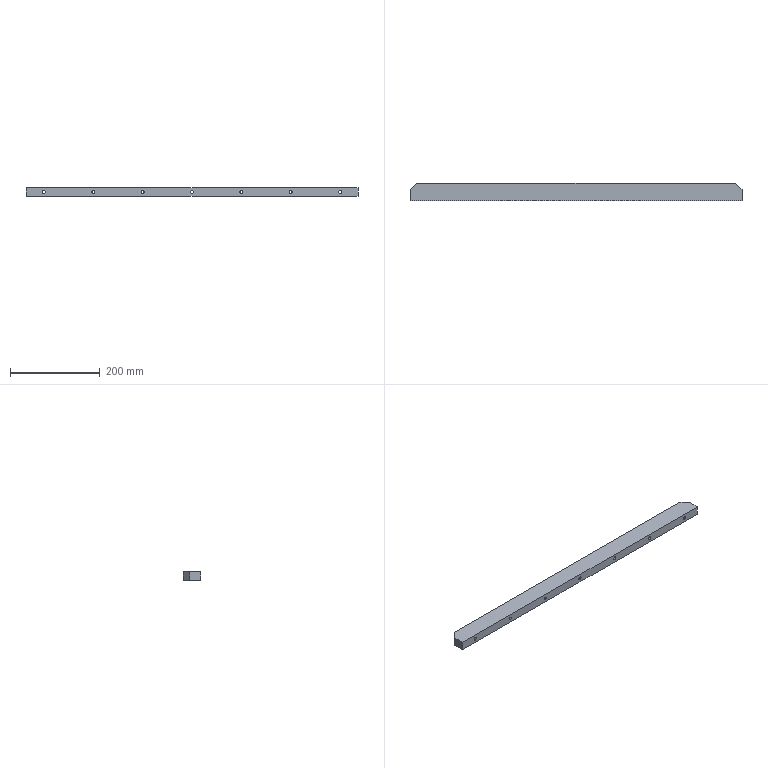Part | SolidWorks | features BaseBody 1 | 1 solid | 43 faces | box 740 x 40 x 20 mm | volume 575026 mm3 | cylinder 28 | plane 15 | commonest cylinder face diameters 6.6 x14 11 x14
STEP:
#1=CARTESIAN_POINT('',(-330.,33.2,-5.5));
#2=VERTEX_POINT('',#1);
#3=CARTESIAN_POINT('',(-330.,33.2,5.5));
#4=VERTEX_POINT('',#3);
#5=CARTESIAN_POINT('',(-330.,33.2,0.));
#6=DIRECTION('',(0.,1.,0.));
#7=DIRECTION('',(0.,0.,1.));
#8=AXIS2_PLACEMENT_3D('',#5,#6,#7);
#9=CIRCLE('',#8,5.5);
#10=EDGE_CURVE('',#2,#4,#9,.T.);
#11=ORIENTED_EDGE('',*,*,#10,.F.);
#12=CARTESIAN_POINT('',(-330.,40.,-5.5));
#13=VERTEX_POINT('',#12);
#14=CARTESIAN_POINT('',(-330.,40.,-5.5));
#15=DIRECTION('',(0.,1.,0.));
#16=VECTOR('',#15,1000.);
#17=LINE('',#14,#16);
#18=EDGE_CURVE('',#2,#13,#17,.T.);
#19=ORIENTED_EDGE('',*,*,#18,.T.);
#20=CARTESIAN_POINT('',(-330.,40.,5.5));
#21=VERTEX_POINT('',#20);
#22=CARTESIAN_POINT('',(-330.,40.,0.));
#23=DIRECTION('',(0.,1.,0.));
#24=DIRECTION('',(0.,0.,1.));
#25=AXIS2_PLACEMENT_3D('',#22,#23,#24);
#26=CIRCLE('',#25,5.5);
#27=EDGE_CURVE('',#13,#21,#26,.T.);
#28=ORIENTED_EDGE('',*,*,#27,.T.);
#29=CARTESIAN_POINT('',(-330.,40.,5.5));
#30=DIRECTION('',(0.,1.,0.));
#31=VECTOR('',#30,1000.);
#32=LINE('',#29,#31);
#33=EDGE_CURVE('',#4,#21,#32,.T.);
#34=ORIENTED_EDGE('',*,*,#33,.F.);
#35=EDGE_LOOP('',(#11,#19,#28,#34));
#36=FACE_OUTER_BOUND('',#35,.T.);
#37=CARTESIAN_POINT('',(-330.,40.,0.));
#38=DIRECTION('',(0.,1.,0.));
#39=DIRECTION('',(0.,0.,1.));
#40=AXIS2_PLACEMENT_3D('',#37,#38,#39);
#41=CYLINDRICAL_SURFACE('',#40,5.5);
#42=ADVANCED_FACE('',(#36),#41,.F.);
#43=CARTESIAN_POINT('',(-330.,0.,3.3));
#44=VERTEX_POINT('',#43);
#45=CARTESIAN_POINT('',(-330.,0.,-3.3));
#46=VERTEX_POINT('',#45);
#47=CARTESIAN_POINT('',(-330.,0.,0.));
#48=DIRECTION('',(0.,-1.,0.));
#49=DIRECTION('',(0.,0.,-1.));
#50=AXIS2_PLACEMENT_3D('',#47,#48,#49);
#51=CIRCLE('',#50,3.3);
#52=EDGE_CURVE('',#44,#46,#51,.T.);
#53=ORIENTED_EDGE('',*,*,#52,.T.);
#54=CARTESIAN_POINT('',(-330.,33.2,-3.3));
#55=VERTEX_POINT('',#54);
#56=CARTESIAN_POINT('',(-330.,40.,-3.3));
#57=DIRECTION('',(0.,1.,0.));
#58=VECTOR('',#57,1000.);
#59=LINE('',#56,#58);
#60=EDGE_CURVE('',#46,#55,#59,.T.);
#61=ORIENTED_EDGE('',*,*,#60,.T.);
#62=CARTESIAN_POINT('',(-330.,33.2,3.3));
#63=VERTEX_POINT('',#62);
#64=CARTESIAN_POINT('',(-330.,33.2,0.));
#65=DIRECTION('',(0.,1.,0.));
#66=DIRECTION('',(0.,0.,1.));
#67=AXIS2_PLACEMENT_3D('',#64,#65,#66);
#68=CIRCLE('',#67,3.3);
#69=EDGE_CURVE('',#55,#63,#68,.T.);
#70=ORIENTED_EDGE('',*,*,#69,.T.);
#71=CARTESIAN_POINT('',(-330.,40.,3.3));
#72=DIRECTION('',(0.,1.,0.));
#73=VECTOR('',#72,1000.);
#74=LINE('',#71,#73);
#75=EDGE_CURVE('',#44,#63,#74,.T.);
#76=ORIENTED_EDGE('',*,*,#75,.F.);
#77=EDGE_LOOP('',(#53,#61,#70,#76));
#78=FACE_OUTER_BOUND('',#77,.T.);
#79=CARTESIAN_POINT('',(-330.,40.,0.));
#80=DIRECTION('',(0.,1.,0.));
#81=DIRECTION('',(0.,0.,1.));
#82=AXIS2_PLACEMENT_3D('',#79,#80,#81);
#83=CYLINDRICAL_SURFACE('',#82,3.3);
#84=ADVANCED_FACE('',(#78),#83,.F.);
#85=CARTESIAN_POINT('',(-220.,33.2,-5.5));
#86=VERTEX_POINT('',#85);
#87=CARTESIAN_POINT('',(-220.,33.2,5.5));
#88=VERTEX_POINT('',#87);
#89=CARTESIAN_POINT('',(-220.,33.2,0.));
#90=DIRECTION('',(0.,1.,0.));
#91=DIRECTION('',(0.,0.,1.));
#92=AXIS2_PLACEMENT_3D('',#89,#90,#91);
#93=CIRCLE('',#92,5.5);
#94=EDGE_CURVE('',#86,#88,#93,.T.);
#95=ORIENTED_EDGE('',*,*,#94,.F.);
#96=CARTESIAN_POINT('',(-220.,40.,-5.5));
#97=VERTEX_POINT('',#96);
#98=CARTESIAN_POINT('',(-220.,40.,-5.5));
#99=DIRECTION('',(0.,1.,0.));
#100=VECTOR('',#99,1000.);
#101=LINE('',#98,#100);
#102=EDGE_CURVE('',#86,#97,#101,.T.);
#103=ORIENTED_EDGE('',*,*,#102,.T.);
#104=CARTESIAN_POINT('',(-220.,40.,5.5));
#105=VERTEX_POINT('',#104);
#106=CARTESIAN_POINT('',(-220.,40.,0.));
#107=DIRECTION('',(0.,1.,0.));
#108=DIRECTION('',(0.,0.,1.));
#109=AXIS2_PLACEMENT_3D('',#106,#107,#108);
#110=CIRCLE('',#109,5.5);
#111=EDGE_CURVE('',#97,#105,#110,.T.);
#112=ORIENTED_EDGE('',*,*,#111,.T.);
#113=CARTESIAN_POINT('',(-220.,40.,5.5));
#114=DIRECTION('',(0.,1.,0.));
#115=VECTOR('',#114,1000.);
#116=LINE('',#113,#115);
#117=EDGE_CURVE('',#88,#105,#116,.T.);
#118=ORIENTED_EDGE('',*,*,#117,.F.);
#119=EDGE_LOOP('',(#95,#103,#112,#118));
#120=FACE_OUTER_BOUND('',#119,.T.);
#121=CARTESIAN_POINT('',(-220.,40.,0.));
#122=DIRECTION('',(0.,1.,0.));
#123=DIRECTION('',(0.,0.,1.));
#124=AXIS2_PLACEMENT_3D('',#121,#122,#123);
#125=CYLINDRICAL_SURFACE('',#124,5.5);
#126=ADVANCED_FACE('',(#120),#125,.F.);
#127=CARTESIAN_POINT('',(-220.,0.,3.3));
#128=VERTEX_POINT('',#127);
#129=CARTESIAN_POINT('',(-220.,0.,-3.3));
#130=VERTEX_POINT('',#129);
#131=CARTESIAN_POINT('',(-220.,0.,0.));
#132=DIRECTION('',(0.,-1.,0.));
#133=DIRECTION('',(0.,0.,-1.));
#134=AXIS2_PLACEMENT_3D('',#131,#132,#133);
#135=CIRCLE('',#134,3.3);
#136=EDGE_CURVE('',#128,#130,#135,.T.);
#137=ORIENTED_EDGE('',*,*,#136,.T.);
#138=CARTESIAN_POINT('',(-220.,33.2,-3.3));
#139=VERTEX_POINT('',#138);
#140=CARTESIAN_POINT('',(-220.,40.,-3.3));
#141=DIRECTION('',(0.,1.,0.));
#142=VECTOR('',#141,1000.);
#143=LINE('',#140,#142);
#144=EDGE_CURVE('',#130,#139,#143,.T.);
#145=ORIENTED_EDGE('',*,*,#144,.T.);
#146=CARTESIAN_POINT('',(-220.,33.2,3.3));
#147=VERTEX_POINT('',#146);
#148=CARTESIAN_POINT('',(-220.,33.2,0.));
#149=DIRECTION('',(0.,1.,0.));
#150=DIRECTION('',(0.,0.,1.));
#151=AXIS2_PLACEMENT_3D('',#148,#149,#150);
#152=CIRCLE('',#151,3.3);
#153=EDGE_CURVE('',#139,#147,#152,.T.);
#154=ORIENTED_EDGE('',*,*,#153,.T.);
#155=CARTESIAN_POINT('',(-220.,40.,3.3));
#156=DIRECTION('',(0.,1.,0.));
#157=VECTOR('',#156,1000.);
#158=LINE('',#155,#157);
#159=EDGE_CURVE('',#128,#147,#158,.T.);
#160=ORIENTED_EDGE('',*,*,#159,.F.);
#161=EDGE_LOOP('',(#137,#145,#154,#160));
#162=FACE_OUTER_BOUND('',#161,.T.);
#163=CARTESIAN_POINT('',(-220.,40.,0.));
#164=DIRECTION('',(0.,1.,0.));
#165=DIRECTION('',(0.,0.,1.));
#166=AXIS2_PLACEMENT_3D('',#163,#164,#165);
#167=CYLINDRICAL_SURFACE('',#166,3.3);
#168=ADVANCED_FACE('',(#162),#167,.F.);
#169=CARTESIAN_POINT('',(-110.,33.2,-5.5));
#170=VERTEX_POINT('',#169);
#171=CARTESIAN_POINT('',(-110.,33.2,5.5));
#172=VERTEX_POINT('',#171);
#173=CARTESIAN_POINT('',(-110.,33.2,0.));
#174=DIRECTION('',(0.,1.,0.));
#175=DIRECTION('',(0.,0.,1.));
#176=AXIS2_PLACEMENT_3D('',#173,#174,#175);
#177=CIRCLE('',#176,5.5);
#178=EDGE_CURVE('',#170,#172,#177,.T.);
#179=ORIENTED_EDGE('',*,*,#178,.F.);
#180=CARTESIAN_POINT('',(-110.,40.,-5.5));
#181=VERTEX_POINT('',#180);
#182=CARTESIAN_POINT('',(-110.,40.,-5.5));
#183=DIRECTION('',(0.,1.,0.));
#184=VECTOR('',#183,1000.);
#185=LINE('',#182,#184);
#186=EDGE_CURVE('',#170,#181,#185,.T.);
#187=ORIENTED_EDGE('',*,*,#186,.T.);
#188=CARTESIAN_POINT('',(-110.,40.,5.5));
#189=VERTEX_POINT('',#188);
#190=CARTESIAN_POINT('',(-110.,40.,0.));
#191=DIRECTION('',(0.,1.,0.));
#192=DIRECTION('',(0.,0.,1.));
#193=AXIS2_PLACEMENT_3D('',#190,#191,#192);
#194=CIRCLE('',#193,5.5);
#195=EDGE_CURVE('',#181,#189,#194,.T.);
#196=ORIENTED_EDGE('',*,*,#195,.T.);
#197=CARTESIAN_POINT('',(-110.,40.,5.5));
#198=DIRECTION('',(0.,1.,0.));
#199=VECTOR('',#198,1000.);
#200=LINE('',#197,#199);
#201=EDGE_CURVE('',#172,#189,#200,.T.);
#202=ORIENTED_EDGE('',*,*,#201,.F.);
#203=EDGE_LOOP('',(#179,#187,#196,#202));
#204=FACE_OUTER_BOUND('',#203,.T.);
#205=CARTESIAN_POINT('',(-110.,40.,0.));
#206=DIRECTION('',(0.,1.,0.));
#207=DIRECTION('',(0.,0.,1.));
#208=AXIS2_PLACEMENT_3D('',#205,#206,#207);
#209=CYLINDRICAL_SURFACE('',#208,5.5);
#210=ADVANCED_FACE('',(#204),#209,.F.);
#211=CARTESIAN_POINT('',(-110.,0.,3.3));
#212=VERTEX_POINT('',#211);
#213=CARTESIAN_POINT('',(-110.,0.,-3.3));
#214=VERTEX_POINT('',#213);
#215=CARTESIAN_POINT('',(-110.,0.,0.));
#216=DIRECTION('',(0.,-1.,0.));
#217=DIRECTION('',(0.,0.,-1.));
#218=AXIS2_PLACEMENT_3D('',#215,#216,#217);
#219=CIRCLE('',#218,3.3);
#220=EDGE_CURVE('',#212,#214,#219,.T.);
#221=ORIENTED_EDGE('',*,*,#220,.T.);
#222=CARTESIAN_POINT('',(-110.,33.2,-3.3));
#223=VERTEX_POINT('',#222);
#224=CARTESIAN_POINT('',(-110.,40.,-3.3));
#225=DIRECTION('',(0.,1.,0.));
#226=VECTOR('',#225,1000.);
#227=LINE('',#224,#226);
#228=EDGE_CURVE('',#214,#223,#227,.T.);
#229=ORIENTED_EDGE('',*,*,#228,.T.);
#230=CARTESIAN_POINT('',(-110.,33.2,3.3));
#231=VERTEX_POINT('',#230);
#232=CARTESIAN_POINT('',(-110.,33.2,0.));
#233=DIRECTION('',(0.,1.,0.));
#234=DIRECTION('',(0.,0.,1.));
#235=AXIS2_PLACEMENT_3D('',#232,#233,#234);
#236=CIRCLE('',#235,3.3);
#237=EDGE_CURVE('',#223,#231,#236,.T.);
#238=ORIENTED_EDGE('',*,*,#237,.T.);
#239=CARTESIAN_POINT('',(-110.,40.,3.3));
#240=DIRECTION('',(0.,1.,0.));
#241=VECTOR('',#240,1000.);
#242=LINE('',#239,#241);
#243=EDGE_CURVE('',#212,#231,#242,.T.);
#244=ORIENTED_EDGE('',*,*,#243,.F.);
#245=EDGE_LOOP('',(#221,#229,#238,#244));
#246=FACE_OUTER_BOUND('',#245,.T.);
#247=CARTESIAN_POINT('',(-110.,40.,0.));
#248=DIRECTION('',(0.,1.,0.));
#249=DIRECTION('',(0.,0.,1.));
#250=AXIS2_PLACEMENT_3D('',#247,#248,#249);
#251=CYLINDRICAL_SURFACE('',#250,3.3);
#252=ADVANCED_FACE('',(#246),#251,.F.);
#253=CARTESIAN_POINT('',(0.,33.2,-5.5));
#254=VERTEX_POINT('',#253);
#255=CARTESIAN_POINT('',(0.,33.2,5.5));
#256=VERTEX_POINT('',#255);
#257=CARTESIAN_POINT('',(0.,33.2,0.));
#258=DIRECTION('',(0.,1.,0.));
#259=DIRECTION('',(0.,0.,1.));
#260=AXIS2_PLACEMENT_3D('',#257,#258,#259);
#261=CIRCLE('',#260,5.5);
#262=EDGE_CURVE('',#254,#256,#261,.T.);
#263=ORIENTED_EDGE('',*,*,#262,.F.);
#264=CARTESIAN_POINT('',(0.,40.,-5.5));
#265=VERTEX_POINT('',#264);
#266=CARTESIAN_POINT('',(0.,40.,-5.5));
#267=DIRECTION('',(0.,1.,0.));
#268=VECTOR('',#267,1000.);
#269=LINE('',#266,#268);
#270=EDGE_CURVE('',#254,#265,#269,.T.);
#271=ORIENTED_EDGE('',*,*,#270,.T.);
#272=CARTESIAN_POINT('',(0.,40.,5.5));
#273=VERTEX_POINT('',#272);
#274=CARTESIAN_POINT('',(0.,40.,0.));
#275=DIRECTION('',(0.,1.,0.));
#276=DIRECTION('',(0.,0.,1.));
#277=AXIS2_PLACEMENT_3D('',#274,#275,#276);
#278=CIRCLE('',#277,5.5);
#279=EDGE_CURVE('',#265,#273,#278,.T.);
#280=ORIENTED_EDGE('',*,*,#279,.T.);
#281=CARTESIAN_POINT('',(0.,40.,5.5));
#282=DIRECTION('',(0.,1.,0.));
#283=VECTOR('',#282,1000.);
#284=LINE('',#281,#283);
#285=EDGE_CURVE('',#256,#273,#284,.T.);
#286=ORIENTED_EDGE('',*,*,#285,.F.);
#287=EDGE_LOOP('',(#263,#271,#280,#286));
#288=FACE_OUTER_BOUND('',#287,.T.);
#289=CARTESIAN_POINT('',(0.,40.,0.));
#290=DIRECTION('',(0.,1.,0.));
#291=DIRECTION('',(0.,0.,1.));
#292=AXIS2_PLACEMENT_3D('',#289,#290,#291);
#293=CYLINDRICAL_SURFACE('',#292,5.5);
#294=ADVANCED_FACE('',(#288),#293,.F.);
#295=CARTESIAN_POINT('',(0.,0.,3.3));
#296=VERTEX_POINT('',#295);
#297=CARTESIAN_POINT('',(0.,0.,-3.3));
#298=VERTEX_POINT('',#297);
#299=CARTESIAN_POINT('',(0.,0.,0.));
#300=DIRECTION('',(0.,-1.,0.));
#301=DIRECTION('',(0.,0.,-1.));
#302=AXIS2_PLACEMENT_3D('',#299,#300,#301);
#303=CIRCLE('',#302,3.3);
#304=EDGE_CURVE('',#296,#298,#303,.T.);
#305=ORIENTED_EDGE('',*,*,#304,.T.);
#306=CARTESIAN_POINT('',(0.,33.2,-3.3));
#307=VERTEX_POINT('',#306);
#308=CARTESIAN_POINT('',(0.,40.,-3.3));
#309=DIRECTION('',(0.,1.,0.));
#310=VECTOR('',#309,1000.);
#311=LINE('',#308,#310);
#312=EDGE_CURVE('',#298,#307,#311,.T.);
#313=ORIENTED_EDGE('',*,*,#312,.T.);
#314=CARTESIAN_POINT('',(0.,33.2,3.3));
#315=VERTEX_POINT('',#314);
#316=CARTESIAN_POINT('',(0.,33.2,0.));
#317=DIRECTION('',(0.,1.,0.));
#318=DIRECTION('',(0.,0.,1.));
#319=AXIS2_PLACEMENT_3D('',#316,#317,#318);
#320=CIRCLE('',#319,3.3);
#321=EDGE_CURVE('',#307,#315,#320,.T.);
#322=ORIENTED_EDGE('',*,*,#321,.T.);
#323=CARTESIAN_POINT('',(0.,40.,3.3));
#324=DIRECTION('',(0.,1.,0.));
#325=VECTOR('',#324,1000.);
#326=LINE('',#323,#325);
#327=EDGE_CURVE('',#296,#315,#326,.T.);
#328=ORIENTED_EDGE('',*,*,#327,.F.);
#329=EDGE_LOOP('',(#305,#313,#322,#328));
#330=FACE_OUTER_BOUND('',#329,.T.);
#331=CARTESIAN_POINT('',(0.,40.,0.));
#332=DIRECTION('',(0.,1.,0.));
#333=DIRECTION('',(0.,0.,1.));
#334=AXIS2_PLACEMENT_3D('',#331,#332,#333);
#335=CYLINDRICAL_SURFACE('',#334,3.3);
#336=ADVANCED_FACE('',(#330),#335,.F.);
#337=CARTESIAN_POINT('',(110.,33.2,-5.5));
#338=VERTEX_POINT('',#337);
#339=CARTESIAN_POINT('',(110.,33.2,5.5));
#340=VERTEX_POINT('',#339);
#341=CARTESIAN_POINT('',(110.,33.2,0.));
#342=DIRECTION('',(0.,1.,0.));
#343=DIRECTION('',(0.,0.,1.));
#344=AXIS2_PLACEMENT_3D('',#341,#342,#343);
#345=CIRCLE('',#344,5.5);
#346=EDGE_CURVE('',#338,#340,#345,.T.);
#347=ORIENTED_EDGE('',*,*,#346,.F.);
#348=CARTESIAN_POINT('',(110.,40.,-5.5));
#349=VERTEX_POINT('',#348);
#350=CARTESIAN_POINT('',(110.,40.,-5.5));
#351=DIRECTION('',(0.,1.,0.));
#352=VECTOR('',#351,1000.);
#353=LINE('',#350,#352);
#354=EDGE_CURVE('',#338,#349,#353,.T.);
#355=ORIENTED_EDGE('',*,*,#354,.T.);
#356=CARTESIAN_POINT('',(110.,40.,5.5));
#357=VERTEX_POINT('',#356);
#358=CARTESIAN_POINT('',(110.,40.,0.));
#359=DIRECTION('',(0.,1.,0.));
#360=DIRECTION('',(0.,0.,1.));
#361=AXIS2_PLACEMENT_3D('',#358,#359,#360);
#362=CIRCLE('',#361,5.5);
#363=EDGE_CURVE('',#349,#357,#362,.T.);
#364=ORIENTED_EDGE('',*,*,#363,.T.);
#365=CARTESIAN_POINT('',(110.,40.,5.5));
#366=DIRECTION('',(0.,1.,0.));
#367=VECTOR('',#366,1000.);
#368=LINE('',#365,#367);
#369=EDGE_CURVE('',#340,#357,#368,.T.);
#370=ORIENTED_EDGE('',*,*,#369,.F.);
#371=EDGE_LOOP('',(#347,#355,#364,#370));
#372=FACE_OUTER_BOUND('',#371,.T.);
#373=CARTESIAN_POINT('',(110.,40.,0.));
#374=DIRECTION('',(0.,1.,0.));
#375=DIRECTION('',(0.,0.,1.));
#376=AXIS2_PLACEMENT_3D('',#373,#374,#375);
#377=CYLINDRICAL_SURFACE('',#376,5.5);
#378=ADVANCED_FACE('',(#372),#377,.F.);
#379=CARTESIAN_POINT('',(110.,0.,3.3));
#380=VERTEX_POINT('',#379);
#381=CARTESIAN_POINT('',(110.,0.,-3.3));
#382=VERTEX_POINT('',#381);
#383=CARTESIAN_POINT('',(110.,0.,0.));
#384=DIRECTION('',(0.,-1.,0.));
#385=DIRECTION('',(0.,0.,-1.));
#386=AXIS2_PLACEMENT_3D('',#383,#384,#385);
#387=CIRCLE('',#386,3.3);
#388=EDGE_CURVE('',#380,#382,#387,.T.);
#389=ORIENTED_EDGE('',*,*,#388,.T.);
#390=CARTESIAN_POINT('',(110.,33.2,-3.3));
#391=VERTEX_POINT('',#390);
#392=CARTESIAN_POINT('',(110.,40.,-3.3));
#393=DIRECTION('',(0.,1.,0.));
#394=VECTOR('',#393,1000.);
#395=LINE('',#392,#394);
#396=EDGE_CURVE('',#382,#391,#395,.T.);
#397=ORIENTED_EDGE('',*,*,#396,.T.);
#398=CARTESIAN_POINT('',(110.,33.2,3.3));
#399=VERTEX_POINT('',#398);
#400=CARTESIAN_POINT('',(110.,33.2,0.));
#401=DIRECTION('',(0.,1.,0.));
#402=DIRECTION('',(0.,0.,1.));
#403=AXIS2_PLACEMENT_3D('',#400,#401,#402);
#404=CIRCLE('',#403,3.3);
#405=EDGE_CURVE('',#391,#399,#404,.T.);
#406=ORIENTED_EDGE('',*,*,#405,.T.);
#407=CARTESIAN_POINT('',(110.,40.,3.3));
#408=DIRECTION('',(0.,1.,0.));
#409=VECTOR('',#408,1000.);
#410=LINE('',#407,#409);
#411=EDGE_CURVE('',#380,#399,#410,.T.);
#412=ORIENTED_EDGE('',*,*,#411,.F.);
#413=EDGE_LOOP('',(#389,#397,#406,#412));
#414=FACE_OUTER_BOUND('',#413,.T.);
#415=CARTESIAN_POINT('',(110.,40.,0.));
#416=DIRECTION('',(0.,1.,0.));
#417=DIRECTION('',(0.,0.,1.));
#418=AXIS2_PLACEMENT_3D('',#415,#416,#417);
#419=CYLINDRICAL_SURFACE('',#418,3.3);
#420=ADVANCED_FACE('',(#414),#419,.F.);
#421=CARTESIAN_POINT('',(220.,33.2,-5.5));
#422=VERTEX_POINT('',#421);
#423=CARTESIAN_POINT('',(220.,33.2,5.5));
#424=VERTEX_POINT('',#423);
#425=CARTESIAN_POINT('',(220.,33.2,0.));
#426=DIRECTION('',(0.,1.,0.));
#427=DIRECTION('',(0.,0.,1.));
#428=AXIS2_PLACEMENT_3D('',#425,#426,#427);
#429=CIRCLE('',#428,5.5);
#430=EDGE_CURVE('',#422,#424,#429,.T.);
#431=ORIENTED_EDGE('',*,*,#430,.F.);
#432=CARTESIAN_POINT('',(220.,40.,-5.5));
#433=VERTEX_POINT('',#432);
#434=CARTESIAN_POINT('',(220.,40.,-5.5));
#435=DIRECTION('',(0.,1.,0.));
#436=VECTOR('',#435,1000.);
#437=LINE('',#434,#436);
#438=EDGE_CURVE('',#422,#433,#437,.T.);
#439=ORIENTED_EDGE('',*,*,#438,.T.);
#440=CARTESIAN_POINT('',(220.,40.,5.5));
#441=VERTEX_POINT('',#440);
#442=CARTESIAN_POINT('',(220.,40.,0.));
#443=DIRECTION('',(0.,1.,0.));
#444=DIRECTION('',(0.,0.,1.));
#445=AXIS2_PLACEMENT_3D('',#442,#443,#444);
#446=CIRCLE('',#445,5.5);
#447=EDGE_CURVE('',#433,#441,#446,.T.);
#448=ORIENTED_EDGE('',*,*,#447,.T.);
#449=CARTESIAN_POINT('',(220.,40.,5.5));
#450=DIRECTION('',(0.,1.,0.));
#451=VECTOR('',#450,1000.);
#452=LINE('',#449,#451);
#453=EDGE_CURVE('',#424,#441,#452,.T.);
#454=ORIENTED_EDGE('',*,*,#453,.F.);
#455=EDGE_LOOP('',(#431,#439,#448,#454));
#456=FACE_OUTER_BOUND('',#455,.T.);
#457=CARTESIAN_POINT('',(220.,40.,0.));
#458=DIRECTION('',(0.,1.,0.));
#459=DIRECTION('',(0.,0.,1.));
#460=AXIS2_PLACEMENT_3D('',#457,#458,#459);
#461=CYLINDRICAL_SURFACE('',#460,5.5);
#462=ADVANCED_FACE('',(#456),#461,.F.);
#463=CARTESIAN_POINT('',(220.,0.,3.3));
#464=VERTEX_POINT('',#463);
#465=CARTESIAN_POINT('',(220.,0.,-3.3));
#466=VERTEX_POINT('',#465);
#467=CARTESIAN_POINT('',(220.,0.,0.));
#468=DIRECTION('',(0.,-1.,0.));
#469=DIRECTION('',(0.,0.,-1.));
#470=AXIS2_PLACEMENT_3D('',#467,#468,#469);
#471=CIRCLE('',#470,3.3);
#472=EDGE_CURVE('',#464,#466,#471,.T.);
#473=ORIENTED_EDGE('',*,*,#472,.T.);
#474=CARTESIAN_POINT('',(220.,33.2,-3.3));
#475=VERTEX_POINT('',#474);
#476=CARTESIAN_POINT('',(220.,40.,-3.3));
#477=DIRECTION('',(0.,1.,0.));
#478=VECTOR('',#477,1000.);
#479=LINE('',#476,#478);
#480=EDGE_CURVE('',#466,#475,#479,.T.);
#481=ORIENTED_EDGE('',*,*,#480,.T.);
#482=CARTESIAN_POINT('',(220.,33.2,3.3));
#483=VERTEX_POINT('',#482);
#484=CARTESIAN_POINT('',(220.,33.2,0.));
#485=DIRECTION('',(0.,1.,0.));
#486=DIRECTION('',(0.,0.,1.));
#487=AXIS2_PLACEMENT_3D('',#484,#485,#486);
#488=CIRCLE('',#487,3.3);
#489=EDGE_CURVE('',#475,#483,#488,.T.);
#490=ORIENTED_EDGE('',*,*,#489,.T.);
#491=CARTESIAN_POINT('',(220.,40.,3.3));
#492=DIRECTION('',(0.,1.,0.));
#493=VECTOR('',#492,1000.);
#494=LINE('',#491,#493);
#495=EDGE_CURVE('',#464,#483,#494,.T.);
#496=ORIENTED_EDGE('',*,*,#495,.F.);
#497=EDGE_LOOP('',(#473,#481,#490,#496));
#498=FACE_OUTER_BOUND('',#497,.T.);
#499=CARTESIAN_POINT('',(220.,40.,0.));
#500=DIRECTION('',(0.,1.,0.));
#501=DIRECTION('',(0.,0.,1.));
#502=AXIS2_PLACEMENT_3D('',#499,#500,#501);
#503=CYLINDRICAL_SURFACE('',#502,3.3);
#504=ADVANCED_FACE('',(#498),#503,.F.);
#505=CARTESIAN_POINT('',(330.,33.2,-5.5));
#506=VERTEX_POINT('',#505);
#507=CARTESIAN_POINT('',(330.,33.2,5.5));
#508=VERTEX_POINT('',#507);
#509=CARTESIAN_POINT('',(330.,33.2,0.));
#510=DIRECTION('',(0.,1.,0.));
#511=DIRECTION('',(0.,0.,1.));
#512=AXIS2_PLACEMENT_3D('',#509,#510,#511);
#513=CIRCLE('',#512,5.5);
#514=EDGE_CURVE('',#506,#508,#513,.T.);
#515=ORIENTED_EDGE('',*,*,#514,.F.);
#516=CARTESIAN_POINT('',(330.,40.,-5.5));
#517=VERTEX_POINT('',#516);
#518=CARTESIAN_POINT('',(330.,40.,-5.5));
#519=DIRECTION('',(0.,1.,0.));
#520=VECTOR('',#519,1000.);
#521=LINE('',#518,#520);
#522=EDGE_CURVE('',#506,#517,#521,.T.);
#523=ORIENTED_EDGE('',*,*,#522,.T.);
#524=CARTESIAN_POINT('',(330.,40.,5.5));
#525=VERTEX_POINT('',#524);
#526=CARTESIAN_POINT('',(330.,40.,0.));
#527=DIRECTION('',(0.,1.,0.));
#528=DIRECTION('',(0.,0.,1.));
#529=AXIS2_PLACEMENT_3D('',#526,#527,#528);
#530=CIRCLE('',#529,5.5);
#531=EDGE_CURVE('',#517,#525,#530,.T.);
#532=ORIENTED_EDGE('',*,*,#531,.T.);
#533=CARTESIAN_POINT('',(330.,40.,5.5));
#534=DIRECTION('',(0.,1.,0.));
#535=VECTOR('',#534,1000.);
#536=LINE('',#533,#535);
#537=EDGE_CURVE('',#508,#525,#536,.T.);
#538=ORIENTED_EDGE('',*,*,#537,.F.);
#539=EDGE_LOOP('',(#515,#523,#532,#538));
#540=FACE_OUTER_BOUND('',#539,.T.);
#541=CARTESIAN_POINT('',(330.,40.,0.));
#542=DIRECTION('',(0.,1.,0.));
#543=DIRECTION('',(0.,0.,1.));
#544=AXIS2_PLACEMENT_3D('',#541,#542,#543);
#545=CYLINDRICAL_SURFACE('',#544,5.5);
#546=ADVANCED_FACE('',(#540),#545,.F.);
#547=CARTESIAN_POINT('',(330.,0.,3.3));
#548=VERTEX_POINT('',#547);
#549=CARTESIAN_POINT('',(330.,0.,-3.3));
#550=VERTEX_POINT('',#549);
#551=CARTESIAN_POINT('',(330.,0.,0.));
#552=DIRECTION('',(0.,-1.,0.));
#553=DIRECTION('',(0.,0.,-1.));
#554=AXIS2_PLACEMENT_3D('',#551,#552,#553);
#555=CIRCLE('',#554,3.3);
#556=EDGE_CURVE('',#548,#550,#555,.T.);
#557=ORIENTED_EDGE('',*,*,#556,.T.);
#558=CARTESIAN_POINT('',(330.,33.2,-3.3));
#559=VERTEX_POINT('',#558);
#560=CARTESIAN_POINT('',(330.,40.,-3.3));
#561=DIRECTION('',(0.,1.,0.));
#562=VECTOR('',#561,1000.);
#563=LINE('',#560,#562);
#564=EDGE_CURVE('',#550,#559,#563,.T.);
#565=ORIENTED_EDGE('',*,*,#564,.T.);
#566=CARTESIAN_POINT('',(330.,33.2,3.3));
#567=VERTEX_POINT('',#566);
#568=CARTESIAN_POINT('',(330.,33.2,0.));
#569=DIRECTION('',(0.,1.,0.));
#570=DIRECTION('',(0.,0.,1.));
#571=AXIS2_PLACEMENT_3D('',#568,#569,#570);
#572=CIRCLE('',#571,3.3);
#573=EDGE_CURVE('',#559,#567,#572,.T.);
#574=ORIENTED_EDGE('',*,*,#573,.T.);
#575=CARTESIAN_POINT('',(330.,40.,3.3));
#576=DIRECTION('',(0.,1.,0.));
#577=VECTOR('',#576,1000.);
#578=LINE('',#575,#577);
#579=EDGE_CURVE('',#548,#567,#578,.T.);
#580=ORIENTED_EDGE('',*,*,#579,.F.);
#581=EDGE_LOOP('',(#557,#565,#574,#580));
#582=FACE_OUTER_BOUND('',#581,.T.);
#583=CARTESIAN_POINT('',(330.,40.,0.));
#584=DIRECTION('',(0.,1.,0.));
#585=DIRECTION('',(0.,0.,1.));
#586=AXIS2_PLACEMENT_3D('',#583,#584,#585);
#587=CYLINDRICAL_SURFACE('',#586,3.3);
#588=ADVANCED_FACE('',(#582),#587,.F.);
#589=CARTESIAN_POINT('',(-370.,25.,-10.));
#590=VERTEX_POINT('',#589);
#591=CARTESIAN_POINT('',(-355.,40.,-10.));
#592=VERTEX_POINT('',#591);
#593=CARTESIAN_POINT('',(-355.,40.,-10.));
#594=DIRECTION('',(0.7071,0.7071,0.));
#595=VECTOR('',#594,1000.);
#596=LINE('',#593,#595);
#597=EDGE_CURVE('',#590,#592,#596,.T.);
#598=ORIENTED_EDGE('',*,*,#597,.F.);
#599=CARTESIAN_POINT('',(-370.,25.,10.));
#600=VERTEX_POINT('',#599);
#601=CARTESIAN_POINT('',(-370.,25.,10.));
#602=DIRECTION('',(0.,0.,-1.));
#603=VECTOR('',#602,1000.);
#604=LINE('',#601,#603);
#605=EDGE_CURVE('',#600,#590,#604,.T.);
#606=ORIENTED_EDGE('',*,*,#605,.F.);
#607=CARTESIAN_POINT('',(-355.,40.,10.));
#608=VERTEX_POINT('',#607);
#609=CARTESIAN_POINT('',(-355.,40.,10.));
#610=DIRECTION('',(-0.7071,-0.7071,0.));
#611=VECTOR('',#610,1000.);
#612=LINE('',#609,#611);
#613=EDGE_CURVE('',#608,#600,#612,.T.);
#614=ORIENTED_EDGE('',*,*,#613,.F.);
#615=CARTESIAN_POINT('',(-355.,40.,0.));
#616=DIRECTION('',(0.,0.,1.));
#617=VECTOR('',#616,1000.);
#618=LINE('',#615,#617);
#619=EDGE_CURVE('',#592,#608,#618,.T.);
#620=ORIENTED_EDGE('',*,*,#619,.F.);
#621=EDGE_LOOP('',(#598,#606,#614,#620));
#622=FACE_OUTER_BOUND('',#621,.T.);
#623=CARTESIAN_POINT('',(-355.,40.,0.));
#624=DIRECTION('',(0.7071,-0.7071,0.));
#625=DIRECTION('',(0.,0.,-1.));
#626=AXIS2_PLACEMENT_3D('',#623,#624,#625);
#627=PLANE('',#626);
#628=ADVANCED_FACE('',(#622),#627,.F.);
#629=CARTESIAN_POINT('',(370.,25.,10.));
#630=VERTEX_POINT('',#629);
#631=CARTESIAN_POINT('',(355.,40.,10.));
#632=VERTEX_POINT('',#631);
#633=CARTESIAN_POINT('',(355.,40.,10.));
#634=DIRECTION('',(-0.7071,0.7071,0.));
#635=VECTOR('',#634,1000.);
#636=LINE('',#633,#635);
#637=EDGE_CURVE('',#630,#632,#636,.T.);
#638=ORIENTED_EDGE('',*,*,#637,.F.);
#639=CARTESIAN_POINT('',(370.,25.,-10.));
#640=VERTEX_POINT('',#639);
#641=CARTESIAN_POINT('',(370.,25.,10.));
#642=DIRECTION('',(0.,0.,1.));
#643=VECTOR('',#642,1000.);
#644=LINE('',#641,#643);
#645=EDGE_CURVE('',#640,#630,#644,.T.);
#646=ORIENTED_EDGE('',*,*,#645,.F.);
#647=CARTESIAN_POINT('',(355.,40.,-10.));
#648=VERTEX_POINT('',#647);
#649=CARTESIAN_POINT('',(355.,40.,-10.));
#650=DIRECTION('',(0.7071,-0.7071,0.));
#651=VECTOR('',#650,1000.);
#652=LINE('',#649,#651);
#653=EDGE_CURVE('',#648,#640,#652,.T.);
#654=ORIENTED_EDGE('',*,*,#653,.F.);
#655=CARTESIAN_POINT('',(355.,40.,0.));
#656=DIRECTION('',(0.,0.,-1.));
#657=VECTOR('',#656,1000.);
#658=LINE('',#655,#657);
#659=EDGE_CURVE('',#632,#648,#658,.T.);
#660=ORIENTED_EDGE('',*,*,#659,.F.);
#661=EDGE_LOOP('',(#638,#646,#654,#660));
#662=FACE_OUTER_BOUND('',#661,.T.);
#663=CARTESIAN_POINT('',(355.,40.,0.));
#664=DIRECTION('',(-0.7071,-0.7071,0.));
#665=DIRECTION('',(-0.7071,0.7071,0.));
#666=AXIS2_PLACEMENT_3D('',#663,#664,#665);
#667=PLANE('',#666);
#668=ADVANCED_FACE('',(#662),#667,.F.);
#669=CARTESIAN_POINT('',(-330.,33.2,0.));
#670=DIRECTION('',(0.,1.,0.));
#671=DIRECTION('',(0.,0.,1.));
#672=AXIS2_PLACEMENT_3D('',#669,#670,#671);
#673=CIRCLE('',#672,3.3);
#674=EDGE_CURVE('',#63,#55,#673,.T.);
#675=ORIENTED_EDGE('',*,*,#674,.F.);
#676=ORIENTED_EDGE('',*,*,#69,.F.);
#677=EDGE_LOOP('',(#675,#676));
#678=FACE_BOUND('',#677,.T.);
#679=CARTESIAN_POINT('',(-330.,33.2,0.));
#680=DIRECTION('',(0.,1.,0.));
#681=DIRECTION('',(0.,0.,1.));
#682=AXIS2_PLACEMENT_3D('',#679,#680,#681);
#683=CIRCLE('',#682,5.5);
#684=EDGE_CURVE('',#4,#2,#683,.T.);
#685=ORIENTED_EDGE('',*,*,#684,.T.);
#686=ORIENTED_EDGE('',*,*,#10,.T.);
#687=EDGE_LOOP('',(#685,#686));
#688=FACE_OUTER_BOUND('',#687,.T.);
#689=CARTESIAN_POINT('',(-326.7,33.2,0.));
#690=DIRECTION('',(0.,-1.,0.));
#691=DIRECTION('',(0.,0.,-1.));
#692=AXIS2_PLACEMENT_3D('',#689,#690,#691);
#693=PLANE('',#692);
#694=ADVANCED_FACE('',(#678,#688),#693,.F.);
#695=CARTESIAN_POINT('',(-220.,33.2,0.));
#696=DIRECTION('',(0.,1.,0.));
#697=DIRECTION('',(0.,0.,1.));
#698=AXIS2_PLACEMENT_3D('',#695,#696,#697);
#699=CIRCLE('',#698,3.3);
#700=EDGE_CURVE('',#147,#139,#699,.T.);
#701=ORIENTED_EDGE('',*,*,#700,.F.);
#702=ORIENTED_EDGE('',*,*,#153,.F.);
#703=EDGE_LOOP('',(#701,#702));
#704=FACE_BOUND('',#703,.T.);
#705=CARTESIAN_POINT('',(-220.,33.2,0.));
#706=DIRECTION('',(0.,1.,0.));
#707=DIRECTION('',(0.,0.,1.));
#708=AXIS2_PLACEMENT_3D('',#705,#706,#707);
#709=CIRCLE('',#708,5.5);
#710=EDGE_CURVE('',#88,#86,#709,.T.);
#711=ORIENTED_EDGE('',*,*,#710,.T.);
#712=ORIENTED_EDGE('',*,*,#94,.T.);
#713=EDGE_LOOP('',(#711,#712));
#714=FACE_OUTER_BOUND('',#713,.T.);
#715=CARTESIAN_POINT('',(-216.7,33.2,0.));
#716=DIRECTION('',(0.,-1.,0.));
#717=DIRECTION('',(0.,0.,-1.));
#718=AXIS2_PLACEMENT_3D('',#715,#716,#717);
#719=PLANE('',#718);
#720=ADVANCED_FACE('',(#704,#714),#719,.F.);
#721=CARTESIAN_POINT('',(-110.,33.2,0.));
#722=DIRECTION('',(0.,1.,0.));
#723=DIRECTION('',(0.,0.,1.));
#724=AXIS2_PLACEMENT_3D('',#721,#722,#723);
#725=CIRCLE('',#724,3.3);
#726=EDGE_CURVE('',#231,#223,#725,.T.);
#727=ORIENTED_EDGE('',*,*,#726,.F.);
#728=ORIENTED_EDGE('',*,*,#237,.F.);
#729=EDGE_LOOP('',(#727,#728));
#730=FACE_BOUND('',#729,.T.);
#731=CARTESIAN_POINT('',(-110.,33.2,0.));
#732=DIRECTION('',(0.,1.,0.));
#733=DIRECTION('',(0.,0.,1.));
#734=AXIS2_PLACEMENT_3D('',#731,#732,#733);
#735=CIRCLE('',#734,5.5);
#736=EDGE_CURVE('',#172,#170,#735,.T.);
#737=ORIENTED_EDGE('',*,*,#736,.T.);
#738=ORIENTED_EDGE('',*,*,#178,.T.);
#739=EDGE_LOOP('',(#737,#738));
#740=FACE_OUTER_BOUND('',#739,.T.);
#741=CARTESIAN_POINT('',(-106.7,33.2,0.));
#742=DIRECTION('',(0.,-1.,0.));
#743=DIRECTION('',(0.,0.,-1.));
#744=AXIS2_PLACEMENT_3D('',#741,#742,#743);
#745=PLANE('',#744);
#746=ADVANCED_FACE('',(#730,#740),#745,.F.);
#747=CARTESIAN_POINT('',(0.,33.2,0.));
#748=DIRECTION('',(0.,1.,0.));
#749=DIRECTION('',(0.,0.,1.));
#750=AXIS2_PLACEMENT_3D('',#747,#748,#749);
#751=CIRCLE('',#750,3.3);
#752=EDGE_CURVE('',#315,#307,#751,.T.);
#753=ORIENTED_EDGE('',*,*,#752,.F.);
#754=ORIENTED_EDGE('',*,*,#321,.F.);
#755=EDGE_LOOP('',(#753,#754));
#756=FACE_BOUND('',#755,.T.);
#757=CARTESIAN_POINT('',(0.,33.2,0.));
#758=DIRECTION('',(0.,1.,0.));
#759=DIRECTION('',(0.,0.,1.));
#760=AXIS2_PLACEMENT_3D('',#757,#758,#759);
#761=CIRCLE('',#760,5.5);
#762=EDGE_CURVE('',#256,#254,#761,.T.);
#763=ORIENTED_EDGE('',*,*,#762,.T.);
#764=ORIENTED_EDGE('',*,*,#262,.T.);
#765=EDGE_LOOP('',(#763,#764));
#766=FACE_OUTER_BOUND('',#765,.T.);
#767=CARTESIAN_POINT('',(3.3,33.2,0.));
#768=DIRECTION('',(0.,-1.,0.));
#769=DIRECTION('',(0.,0.,-1.));
#770=AXIS2_PLACEMENT_3D('',#767,#768,#769);
#771=PLANE('',#770);
#772=ADVANCED_FACE('',(#756,#766),#771,.F.);
#773=CARTESIAN_POINT('',(110.,33.2,0.));
#774=DIRECTION('',(0.,1.,0.));
#775=DIRECTION('',(0.,0.,1.));
#776=AXIS2_PLACEMENT_3D('',#773,#774,#775);
#777=CIRCLE('',#776,3.3);
#778=EDGE_CURVE('',#399,#391,#777,.T.);
#779=ORIENTED_EDGE('',*,*,#778,.F.);
#780=ORIENTED_EDGE('',*,*,#405,.F.);
#781=EDGE_LOOP('',(#779,#780));
#782=FACE_BOUND('',#781,.T.);
#783=CARTESIAN_POINT('',(110.,33.2,0.));
#784=DIRECTION('',(0.,1.,0.));
#785=DIRECTION('',(0.,0.,1.));
#786=AXIS2_PLACEMENT_3D('',#783,#784,#785);
#787=CIRCLE('',#786,5.5);
#788=EDGE_CURVE('',#340,#338,#787,.T.);
#789=ORIENTED_EDGE('',*,*,#788,.T.);
#790=ORIENTED_EDGE('',*,*,#346,.T.);
#791=EDGE_LOOP('',(#789,#790));
#792=FACE_OUTER_BOUND('',#791,.T.);
#793=CARTESIAN_POINT('',(113.3,33.2,0.));
#794=DIRECTION('',(0.,-1.,0.));
#795=DIRECTION('',(0.,0.,-1.));
#796=AXIS2_PLACEMENT_3D('',#793,#794,#795);
#797=PLANE('',#796);
#798=ADVANCED_FACE('',(#782,#792),#797,.F.);
#799=CARTESIAN_POINT('',(220.,33.2,0.));
#800=DIRECTION('',(0.,1.,0.));
#801=DIRECTION('',(0.,0.,1.));
#802=AXIS2_PLACEMENT_3D('',#799,#800,#801);
#803=CIRCLE('',#802,3.3);
#804=EDGE_CURVE('',#483,#475,#803,.T.);
#805=ORIENTED_EDGE('',*,*,#804,.F.);
#806=ORIENTED_EDGE('',*,*,#489,.F.);
#807=EDGE_LOOP('',(#805,#806));
#808=FACE_BOUND('',#807,.T.);
#809=CARTESIAN_POINT('',(220.,33.2,0.));
#810=DIRECTION('',(0.,1.,0.));
#811=DIRECTION('',(0.,0.,1.));
#812=AXIS2_PLACEMENT_3D('',#809,#810,#811);
#813=CIRCLE('',#812,5.5);
#814=EDGE_CURVE('',#424,#422,#813,.T.);
#815=ORIENTED_EDGE('',*,*,#814,.T.);
#816=ORIENTED_EDGE('',*,*,#430,.T.);
#817=EDGE_LOOP('',(#815,#816));
#818=FACE_OUTER_BOUND('',#817,.T.);
#819=CARTESIAN_POINT('',(223.3,33.2,0.));
#820=DIRECTION('',(0.,-1.,0.));
#821=DIRECTION('',(0.,0.,-1.));
#822=AXIS2_PLACEMENT_3D('',#819,#820,#821);
#823=PLANE('',#822);
#824=ADVANCED_FACE('',(#808,#818),#823,.F.);
#825=CARTESIAN_POINT('',(330.,33.2,0.));
#826=DIRECTION('',(0.,1.,0.));
#827=DIRECTION('',(0.,0.,1.));
#828=AXIS2_PLACEMENT_3D('',#825,#826,#827);
#829=CIRCLE('',#828,3.3);
#830=EDGE_CURVE('',#567,#559,#829,.T.);
#831=ORIENTED_EDGE('',*,*,#830,.F.);
#832=ORIENTED_EDGE('',*,*,#573,.F.);
#833=EDGE_LOOP('',(#831,#832));
#834=FACE_BOUND('',#833,.T.);
#835=CARTESIAN_POINT('',(330.,33.2,0.));
#836=DIRECTION('',(0.,1.,0.));
#837=DIRECTION('',(0.,0.,1.));
#838=AXIS2_PLACEMENT_3D('',#835,#836,#837);
#839=CIRCLE('',#838,5.5);
#840=EDGE_CURVE('',#508,#506,#839,.T.);
#841=ORIENTED_EDGE('',*,*,#840,.T.);
#842=ORIENTED_EDGE('',*,*,#514,.T.);
#843=EDGE_LOOP('',(#841,#842));
#844=FACE_OUTER_BOUND('',#843,.T.);
#845=CARTESIAN_POINT('',(333.3,33.2,0.));
#846=DIRECTION('',(0.,-1.,0.));
#847=DIRECTION('',(0.,0.,-1.));
#848=AXIS2_PLACEMENT_3D('',#845,#846,#847);
#849=PLANE('',#848);
#850=ADVANCED_FACE('',(#834,#844),#849,.F.);
#851=ORIENTED_EDGE('',*,*,#556,.F.);
#852=CARTESIAN_POINT('',(330.,0.,0.));
#853=DIRECTION('',(0.,-1.,0.));
#854=DIRECTION('',(0.,0.,-1.));
#855=AXIS2_PLACEMENT_3D('',#852,#853,#854);
#856=CIRCLE('',#855,3.3);
#857=EDGE_CURVE('',#550,#548,#856,.T.);
#858=ORIENTED_EDGE('',*,*,#857,.F.);
#859=EDGE_LOOP('',(#851,#858));
#860=FACE_BOUND('',#859,.T.);
#861=ORIENTED_EDGE('',*,*,#472,.F.);
#862=CARTESIAN_POINT('',(220.,0.,0.));
#863=DIRECTION('',(0.,-1.,0.));
#864=DIRECTION('',(0.,0.,-1.));
#865=AXIS2_PLACEMENT_3D('',#862,#863,#864);
#866=CIRCLE('',#865,3.3);
#867=EDGE_CURVE('',#466,#464,#866,.T.);
#868=ORIENTED_EDGE('',*,*,#867,.F.);
#869=EDGE_LOOP('',(#861,#868));
#870=FACE_BOUND('',#869,.T.);
#871=ORIENTED_EDGE('',*,*,#388,.F.);
#872=CARTESIAN_POINT('',(110.,0.,0.));
#873=DIRECTION('',(0.,-1.,0.));
#874=DIRECTION('',(0.,0.,-1.));
#875=AXIS2_PLACEMENT_3D('',#872,#873,#874);
#876=CIRCLE('',#875,3.3);
#877=EDGE_CURVE('',#382,#380,#876,.T.);
#878=ORIENTED_EDGE('',*,*,#877,.F.);
#879=EDGE_LOOP('',(#871,#878));
#880=FACE_BOUND('',#879,.T.);
#881=ORIENTED_EDGE('',*,*,#304,.F.);
#882=CARTESIAN_POINT('',(0.,0.,0.));
#883=DIRECTION('',(0.,-1.,0.));
#884=DIRECTION('',(0.,0.,-1.));
#885=AXIS2_PLACEMENT_3D('',#882,#883,#884);
#886=CIRCLE('',#885,3.3);
#887=EDGE_CURVE('',#298,#296,#886,.T.);
#888=ORIENTED_EDGE('',*,*,#887,.F.);
#889=EDGE_LOOP('',(#881,#888));
#890=FACE_BOUND('',#889,.T.);
#891=ORIENTED_EDGE('',*,*,#220,.F.);
#892=CARTESIAN_POINT('',(-110.,0.,0.));
#893=DIRECTION('',(0.,-1.,0.));
#894=DIRECTION('',(0.,0.,-1.));
#895=AXIS2_PLACEMENT_3D('',#892,#893,#894);
#896=CIRCLE('',#895,3.3);
#897=EDGE_CURVE('',#214,#212,#896,.T.);
#898=ORIENTED_EDGE('',*,*,#897,.F.);
#899=EDGE_LOOP('',(#891,#898));
#900=FACE_BOUND('',#899,.T.);
#901=ORIENTED_EDGE('',*,*,#136,.F.);
#902=CARTESIAN_POINT('',(-220.,0.,0.));
#903=DIRECTION('',(0.,-1.,0.));
#904=DIRECTION('',(0.,0.,-1.));
#905=AXIS2_PLACEMENT_3D('',#902,#903,#904);
#906=CIRCLE('',#905,3.3);
#907=EDGE_CURVE('',#130,#128,#906,.T.);
#908=ORIENTED_EDGE('',*,*,#907,.F.);
#909=EDGE_LOOP('',(#901,#908));
#910=FACE_BOUND('',#909,.T.);
#911=ORIENTED_EDGE('',*,*,#52,.F.);
#912=CARTESIAN_POINT('',(-330.,0.,0.));
#913=DIRECTION('',(0.,-1.,0.));
#914=DIRECTION('',(0.,0.,-1.));
#915=AXIS2_PLACEMENT_3D('',#912,#913,#914);
#916=CIRCLE('',#915,3.3);
#917=EDGE_CURVE('',#46,#44,#916,.T.);
#918=ORIENTED_EDGE('',*,*,#917,.F.);
#919=EDGE_LOOP('',(#911,#918));
#920=FACE_BOUND('',#919,.T.);
#921=CARTESIAN_POINT('',(370.,0.,10.));
#922=VERTEX_POINT('',#921);
#923=CARTESIAN_POINT('',(370.,0.,-10.));
#924=VERTEX_POINT('',#923);
#925=CARTESIAN_POINT('',(370.,0.,10.));
#926=DIRECTION('',(0.,0.,-1.));
#927=VECTOR('',#926,1000.);
#928=LINE('',#925,#927);
#929=EDGE_CURVE('',#922,#924,#928,.T.);
#930=ORIENTED_EDGE('',*,*,#929,.F.);
#931=CARTESIAN_POINT('',(-370.,0.,10.));
#932=VERTEX_POINT('',#931);
#933=CARTESIAN_POINT('',(-370.,0.,10.));
#934=DIRECTION('',(1.,0.,0.));
#935=VECTOR('',#934,1000.);
#936=LINE('',#933,#935);
#937=EDGE_CURVE('',#932,#922,#936,.T.);
#938=ORIENTED_EDGE('',*,*,#937,.F.);
#939=CARTESIAN_POINT('',(-370.,0.,-10.));
#940=VERTEX_POINT('',#939);
#941=CARTESIAN_POINT('',(-370.,0.,10.));
#942=DIRECTION('',(0.,0.,1.));
#943=VECTOR('',#942,1000.);
#944=LINE('',#941,#943);
#945=EDGE_CURVE('',#940,#932,#944,.T.);
#946=ORIENTED_EDGE('',*,*,#945,.F.);
#947=CARTESIAN_POINT('',(-370.,0.,-10.));
#948=DIRECTION('',(-1.,0.,0.));
#949=VECTOR('',#948,1000.);
#950=LINE('',#947,#949);
#951=EDGE_CURVE('',#924,#940,#950,.T.);
#952=ORIENTED_EDGE('',*,*,#951,.F.);
#953=EDGE_LOOP('',(#930,#938,#946,#952));
#954=FACE_OUTER_BOUND('',#953,.T.);
#955=CARTESIAN_POINT('',(0.,0.,0.));
#956=DIRECTION('',(0.,-1.,0.));
#957=DIRECTION('',(0.,0.,-1.));
#958=AXIS2_PLACEMENT_3D('',#955,#956,#957);
#959=PLANE('',#958);
#960=ADVANCED_FACE('',(#860,#870,#880,#890,#900,#910,#920,#954),#959,.T.);
#961=CARTESIAN_POINT('',(330.,40.,0.));
#962=DIRECTION('',(0.,1.,0.));
#963=DIRECTION('',(0.,0.,1.));
#964=AXIS2_PLACEMENT_3D('',#961,#962,#963);
#965=CIRCLE('',#964,5.5);
#966=EDGE_CURVE('',#525,#517,#965,.T.);
#967=ORIENTED_EDGE('',*,*,#966,.F.);
#968=ORIENTED_EDGE('',*,*,#531,.F.);
#969=EDGE_LOOP('',(#967,#968));
#970=FACE_BOUND('',#969,.T.);
#971=CARTESIAN_POINT('',(220.,40.,0.));
#972=DIRECTION('',(0.,1.,0.));
#973=DIRECTION('',(0.,0.,1.));
#974=AXIS2_PLACEMENT_3D('',#971,#972,#973);
#975=CIRCLE('',#974,5.5);
#976=EDGE_CURVE('',#441,#433,#975,.T.);
#977=ORIENTED_EDGE('',*,*,#976,.F.);
#978=ORIENTED_EDGE('',*,*,#447,.F.);
#979=EDGE_LOOP('',(#977,#978));
#980=FACE_BOUND('',#979,.T.);
#981=CARTESIAN_POINT('',(110.,40.,0.));
#982=DIRECTION('',(0.,1.,0.));
#983=DIRECTION('',(0.,0.,1.));
#984=AXIS2_PLACEMENT_3D('',#981,#982,#983);
#985=CIRCLE('',#984,5.5);
#986=EDGE_CURVE('',#357,#349,#985,.T.);
#987=ORIENTED_EDGE('',*,*,#986,.F.);
#988=ORIENTED_EDGE('',*,*,#363,.F.);
#989=EDGE_LOOP('',(#987,#988));
#990=FACE_BOUND('',#989,.T.);
#991=CARTESIAN_POINT('',(0.,40.,0.));
#992=DIRECTION('',(0.,1.,0.));
#993=DIRECTION('',(0.,0.,1.));
#994=AXIS2_PLACEMENT_3D('',#991,#992,#993);
#995=CIRCLE('',#994,5.5);
#996=EDGE_CURVE('',#273,#265,#995,.T.);
#997=ORIENTED_EDGE('',*,*,#996,.F.);
#998=ORIENTED_EDGE('',*,*,#279,.F.);
#999=EDGE_LOOP('',(#997,#998));
#1000=FACE_BOUND('',#999,.T.);
#1001=CARTESIAN_POINT('',(-110.,40.,0.));
#1002=DIRECTION('',(0.,1.,0.));
#1003=DIRECTION('',(0.,0.,1.));
#1004=AXIS2_PLACEMENT_3D('',#1001,#1002,#1003);
#1005=CIRCLE('',#1004,5.5);
#1006=EDGE_CURVE('',#189,#181,#1005,.T.);
#1007=ORIENTED_EDGE('',*,*,#1006,.F.);
#1008=ORIENTED_EDGE('',*,*,#195,.F.);
#1009=EDGE_LOOP('',(#1007,#1008));
#1010=FACE_BOUND('',#1009,.T.);
#1011=CARTESIAN_POINT('',(-220.,40.,0.));
#1012=DIRECTION('',(0.,1.,0.));
#1013=DIRECTION('',(0.,0.,1.));
#1014=AXIS2_PLACEMENT_3D('',#1011,#1012,#1013);
#1015=CIRCLE('',#1014,5.5);
#1016=EDGE_CURVE('',#105,#97,#1015,.T.);
#1017=ORIENTED_EDGE('',*,*,#1016,.F.);
#1018=ORIENTED_EDGE('',*,*,#111,.F.);
#1019=EDGE_LOOP('',(#1017,#1018));
#1020=FACE_BOUND('',#1019,.T.);
#1021=CARTESIAN_POINT('',(-330.,40.,0.));
#1022=DIRECTION('',(0.,1.,0.));
#1023=DIRECTION('',(0.,0.,1.));
#1024=AXIS2_PLACEMENT_3D('',#1021,#1022,#1023);
#1025=CIRCLE('',#1024,5.5);
#1026=EDGE_CURVE('',#21,#13,#1025,.T.);
#1027=ORIENTED_EDGE('',*,*,#1026,.F.);
#1028=ORIENTED_EDGE('',*,*,#27,.F.);
#1029=EDGE_LOOP('',(#1027,#1028));
#1030=FACE_BOUND('',#1029,.T.);
#1031=CARTESIAN_POINT('',(-370.,40.,10.));
#1032=DIRECTION('',(1.,0.,0.));
#1033=VECTOR('',#1032,1000.);
#1034=LINE('',#1031,#1033);
#1035=EDGE_CURVE('',#608,#632,#1034,.T.);
#1036=ORIENTED_EDGE('',*,*,#1035,.T.);
#1037=ORIENTED_EDGE('',*,*,#659,.T.);
#1038=CARTESIAN_POINT('',(-370.,40.,-10.));
#1039=DIRECTION('',(-1.,0.,0.));
#1040=VECTOR('',#1039,1000.);
#1041=LINE('',#1038,#1040);
#1042=EDGE_CURVE('',#648,#592,#1041,.T.);
#1043=ORIENTED_EDGE('',*,*,#1042,.T.);
#1044=ORIENTED_EDGE('',*,*,#619,.T.);
#1045=EDGE_LOOP('',(#1036,#1037,#1043,#1044));
#1046=FACE_OUTER_BOUND('',#1045,.T.);
#1047=CARTESIAN_POINT('',(0.,40.,0.));
#1048=DIRECTION('',(0.,-1.,0.));
#1049=DIRECTION('',(0.,0.,-1.));
#1050=AXIS2_PLACEMENT_3D('',#1047,#1048,#1049);
#1051=PLANE('',#1050);
#1052=ADVANCED_FACE('',(#970,#980,#990,#1000,#1010,#1020,#1030,#1046),#1051,.F.);
#1053=CARTESIAN_POINT('',(370.,40.,10.));
#1054=DIRECTION('',(0.,-1.,0.));
#1055=VECTOR('',#1054,1000.);
#1056=LINE('',#1053,#1055);
#1057=EDGE_CURVE('',#630,#922,#1056,.T.);
#1058=ORIENTED_EDGE('',*,*,#1057,.F.);
#1059=ORIENTED_EDGE('',*,*,#637,.T.);
#1060=ORIENTED_EDGE('',*,*,#1035,.F.);
#1061=ORIENTED_EDGE('',*,*,#613,.T.);
#1062=CARTESIAN_POINT('',(-370.,40.,10.));
#1063=DIRECTION('',(0.,-1.,0.));
#1064=VECTOR('',#1063,1000.);
#1065=LINE('',#1062,#1064);
#1066=EDGE_CURVE('',#600,#932,#1065,.T.);
#1067=ORIENTED_EDGE('',*,*,#1066,.T.);
#1068=ORIENTED_EDGE('',*,*,#937,.T.);
#1069=EDGE_LOOP('',(#1058,#1059,#1060,#1061,#1067,#1068));
#1070=FACE_OUTER_BOUND('',#1069,.T.);
#1071=CARTESIAN_POINT('',(-370.,40.,10.));
#1072=DIRECTION('',(0.,0.,-1.));
#1073=DIRECTION('',(0.,-1.,0.));
#1074=AXIS2_PLACEMENT_3D('',#1071,#1072,#1073);
#1075=PLANE('',#1074);
#1076=ADVANCED_FACE('',(#1070),#1075,.F.);
#1077=ORIENTED_EDGE('',*,*,#1066,.F.);
#1078=ORIENTED_EDGE('',*,*,#605,.T.);
#1079=CARTESIAN_POINT('',(-370.,40.,-10.));
#1080=DIRECTION('',(0.,-1.,0.));
#1081=VECTOR('',#1080,1000.);
#1082=LINE('',#1079,#1081);
#1083=EDGE_CURVE('',#590,#940,#1082,.T.);
#1084=ORIENTED_EDGE('',*,*,#1083,.T.);
#1085=ORIENTED_EDGE('',*,*,#945,.T.);
#1086=EDGE_LOOP('',(#1077,#1078,#1084,#1085));
#1087=FACE_OUTER_BOUND('',#1086,.T.);
#1088=CARTESIAN_POINT('',(-370.,40.,10.));
#1089=DIRECTION('',(1.,0.,0.));
#1090=DIRECTION('',(0.,1.,0.));
#1091=AXIS2_PLACEMENT_3D('',#1088,#1089,#1090);
#1092=PLANE('',#1091);
#1093=ADVANCED_FACE('',(#1087),#1092,.F.);
#1094=ORIENTED_EDGE('',*,*,#1042,.F.);
#1095=ORIENTED_EDGE('',*,*,#653,.T.);
#1096=CARTESIAN_POINT('',(370.,40.,-10.));
#1097=DIRECTION('',(0.,-1.,0.));
#1098=VECTOR('',#1097,1000.);
#1099=LINE('',#1096,#1098);
#1100=EDGE_CURVE('',#640,#924,#1099,.T.);
#1101=ORIENTED_EDGE('',*,*,#1100,.T.);
#1102=ORIENTED_EDGE('',*,*,#951,.T.);
#1103=ORIENTED_EDGE('',*,*,#1083,.F.);
#1104=ORIENTED_EDGE('',*,*,#597,.T.);
#1105=EDGE_LOOP('',(#1094,#1095,#1101,#1102,#1103,#1104));
#1106=FACE_OUTER_BOUND('',#1105,.T.);
#1107=CARTESIAN_POINT('',(-370.,40.,-10.));
#1108=DIRECTION('',(0.,0.,1.));
#1109=DIRECTION('',(1.,0.,0.));
#1110=AXIS2_PLACEMENT_3D('',#1107,#1108,#1109);
#1111=PLANE('',#1110);
#1112=ADVANCED_FACE('',(#1106),#1111,.F.);
#1113=ORIENTED_EDGE('',*,*,#1100,.F.);
#1114=ORIENTED_EDGE('',*,*,#645,.T.);
#1115=ORIENTED_EDGE('',*,*,#1057,.T.);
#1116=ORIENTED_EDGE('',*,*,#929,.T.);
#1117=EDGE_LOOP('',(#1113,#1114,#1115,#1116));
#1118=FACE_OUTER_BOUND('',#1117,.T.);
#1119=CARTESIAN_POINT('',(370.,40.,10.));
#1120=DIRECTION('',(-1.,0.,0.));
#1121=DIRECTION('',(0.,0.,1.));
#1122=AXIS2_PLACEMENT_3D('',#1119,#1120,#1121);
#1123=PLANE('',#1122);
#1124=ADVANCED_FACE('',(#1118),#1123,.F.);
#1125=ORIENTED_EDGE('',*,*,#564,.F.);
#1126=ORIENTED_EDGE('',*,*,#857,.T.);
#1127=ORIENTED_EDGE('',*,*,#579,.T.);
#1128=ORIENTED_EDGE('',*,*,#830,.T.);
#1129=EDGE_LOOP('',(#1125,#1126,#1127,#1128));
#1130=FACE_OUTER_BOUND('',#1129,.T.);
#1131=CARTESIAN_POINT('',(330.,40.,0.));
#1132=DIRECTION('',(0.,1.,0.));
#1133=DIRECTION('',(0.,0.,1.));
#1134=AXIS2_PLACEMENT_3D('',#1131,#1132,#1133);
#1135=CYLINDRICAL_SURFACE('',#1134,3.3);
#1136=ADVANCED_FACE('',(#1130),#1135,.F.);
#1137=ORIENTED_EDGE('',*,*,#522,.F.);
#1138=ORIENTED_EDGE('',*,*,#840,.F.);
#1139=ORIENTED_EDGE('',*,*,#537,.T.);
#1140=ORIENTED_EDGE('',*,*,#966,.T.);
#1141=EDGE_LOOP('',(#1137,#1138,#1139,#1140));
#1142=FACE_OUTER_BOUND('',#1141,.T.);
#1143=CARTESIAN_POINT('',(330.,40.,0.));
#1144=DIRECTION('',(0.,1.,0.));
#1145=DIRECTION('',(0.,0.,1.));
#1146=AXIS2_PLACEMENT_3D('',#1143,#1144,#1145);
#1147=CYLINDRICAL_SURFACE('',#1146,5.5);
#1148=ADVANCED_FACE('',(#1142),#1147,.F.);
#1149=ORIENTED_EDGE('',*,*,#480,.F.);
#1150=ORIENTED_EDGE('',*,*,#867,.T.);
#1151=ORIENTED_EDGE('',*,*,#495,.T.);
#1152=ORIENTED_EDGE('',*,*,#804,.T.);
#1153=EDGE_LOOP('',(#1149,#1150,#1151,#1152));
#1154=FACE_OUTER_BOUND('',#1153,.T.);
#1155=CARTESIAN_POINT('',(220.,40.,0.));
#1156=DIRECTION('',(0.,1.,0.));
#1157=DIRECTION('',(0.,0.,1.));
#1158=AXIS2_PLACEMENT_3D('',#1155,#1156,#1157);
#1159=CYLINDRICAL_SURFACE('',#1158,3.3);
#1160=ADVANCED_FACE('',(#1154),#1159,.F.);
#1161=ORIENTED_EDGE('',*,*,#438,.F.);
#1162=ORIENTED_EDGE('',*,*,#814,.F.);
#1163=ORIENTED_EDGE('',*,*,#453,.T.);
#1164=ORIENTED_EDGE('',*,*,#976,.T.);
#1165=EDGE_LOOP('',(#1161,#1162,#1163,#1164));
#1166=FACE_OUTER_BOUND('',#1165,.T.);
#1167=CARTESIAN_POINT('',(220.,40.,0.));
#1168=DIRECTION('',(0.,1.,0.));
#1169=DIRECTION('',(0.,0.,1.));
#1170=AXIS2_PLACEMENT_3D('',#1167,#1168,#1169);
#1171=CYLINDRICAL_SURFACE('',#1170,5.5);
#1172=ADVANCED_FACE('',(#1166),#1171,.F.);
#1173=ORIENTED_EDGE('',*,*,#396,.F.);
#1174=ORIENTED_EDGE('',*,*,#877,.T.);
#1175=ORIENTED_EDGE('',*,*,#411,.T.);
#1176=ORIENTED_EDGE('',*,*,#778,.T.);
#1177=EDGE_LOOP('',(#1173,#1174,#1175,#1176));
#1178=FACE_OUTER_BOUND('',#1177,.T.);
#1179=CARTESIAN_POINT('',(110.,40.,0.));
#1180=DIRECTION('',(0.,1.,0.));
#1181=DIRECTION('',(0.,0.,1.));
#1182=AXIS2_PLACEMENT_3D('',#1179,#1180,#1181);
#1183=CYLINDRICAL_SURFACE('',#1182,3.3);
#1184=ADVANCED_FACE('',(#1178),#1183,.F.);
#1185=ORIENTED_EDGE('',*,*,#354,.F.);
#1186=ORIENTED_EDGE('',*,*,#788,.F.);
#1187=ORIENTED_EDGE('',*,*,#369,.T.);
#1188=ORIENTED_EDGE('',*,*,#986,.T.);
#1189=EDGE_LOOP('',(#1185,#1186,#1187,#1188));
#1190=FACE_OUTER_BOUND('',#1189,.T.);
#1191=CARTESIAN_POINT('',(110.,40.,0.));
#1192=DIRECTION('',(0.,1.,0.));
#1193=DIRECTION('',(0.,0.,1.));
#1194=AXIS2_PLACEMENT_3D('',#1191,#1192,#1193);
#1195=CYLINDRICAL_SURFACE('',#1194,5.5);
#1196=ADVANCED_FACE('',(#1190),#1195,.F.);
#1197=ORIENTED_EDGE('',*,*,#312,.F.);
#1198=ORIENTED_EDGE('',*,*,#887,.T.);
#1199=ORIENTED_EDGE('',*,*,#327,.T.);
#1200=ORIENTED_EDGE('',*,*,#752,.T.);
#1201=EDGE_LOOP('',(#1197,#1198,#1199,#1200));
#1202=FACE_OUTER_BOUND('',#1201,.T.);
#1203=CARTESIAN_POINT('',(0.,40.,0.));
#1204=DIRECTION('',(0.,1.,0.));
#1205=DIRECTION('',(0.,0.,1.));
#1206=AXIS2_PLACEMENT_3D('',#1203,#1204,#1205);
#1207=CYLINDRICAL_SURFACE('',#1206,3.3);
#1208=ADVANCED_FACE('',(#1202),#1207,.F.);
#1209=ORIENTED_EDGE('',*,*,#270,.F.);
#1210=ORIENTED_EDGE('',*,*,#762,.F.);
#1211=ORIENTED_EDGE('',*,*,#285,.T.);
#1212=ORIENTED_EDGE('',*,*,#996,.T.);
#1213=EDGE_LOOP('',(#1209,#1210,#1211,#1212));
#1214=FACE_OUTER_BOUND('',#1213,.T.);
#1215=CARTESIAN_POINT('',(0.,40.,0.));
#1216=DIRECTION('',(0.,1.,0.));
#1217=DIRECTION('',(0.,0.,1.));
#1218=AXIS2_PLACEMENT_3D('',#1215,#1216,#1217);
#1219=CYLINDRICAL_SURFACE('',#1218,5.5);
#1220=ADVANCED_FACE('',(#1214),#1219,.F.);
#1221=ORIENTED_EDGE('',*,*,#228,.F.);
#1222=ORIENTED_EDGE('',*,*,#897,.T.);
#1223=ORIENTED_EDGE('',*,*,#243,.T.);
#1224=ORIENTED_EDGE('',*,*,#726,.T.);
#1225=EDGE_LOOP('',(#1221,#1222,#1223,#1224));
#1226=FACE_OUTER_BOUND('',#1225,.T.);
#1227=CARTESIAN_POINT('',(-110.,40.,0.));
#1228=DIRECTION('',(0.,1.,0.));
#1229=DIRECTION('',(0.,0.,1.));
#1230=AXIS2_PLACEMENT_3D('',#1227,#1228,#1229);
#1231=CYLINDRICAL_SURFACE('',#1230,3.3);
#1232=ADVANCED_FACE('',(#1226),#1231,.F.);
#1233=ORIENTED_EDGE('',*,*,#186,.F.);
#1234=ORIENTED_EDGE('',*,*,#736,.F.);
#1235=ORIENTED_EDGE('',*,*,#201,.T.);
#1236=ORIENTED_EDGE('',*,*,#1006,.T.);
#1237=EDGE_LOOP('',(#1233,#1234,#1235,#1236));
#1238=FACE_OUTER_BOUND('',#1237,.T.);
#1239=CARTESIAN_POINT('',(-110.,40.,0.));
#1240=DIRECTION('',(0.,1.,0.));
#1241=DIRECTION('',(0.,0.,1.));
#1242=AXIS2_PLACEMENT_3D('',#1239,#1240,#1241);
#1243=CYLINDRICAL_SURFACE('',#1242,5.5);
#1244=ADVANCED_FACE('',(#1238),#1243,.F.);
#1245=ORIENTED_EDGE('',*,*,#144,.F.);
#1246=ORIENTED_EDGE('',*,*,#907,.T.);
#1247=ORIENTED_EDGE('',*,*,#159,.T.);
#1248=ORIENTED_EDGE('',*,*,#700,.T.);
#1249=EDGE_LOOP('',(#1245,#1246,#1247,#1248));
#1250=FACE_OUTER_BOUND('',#1249,.T.);
#1251=CARTESIAN_POINT('',(-220.,40.,0.));
#1252=DIRECTION('',(0.,1.,0.));
#1253=DIRECTION('',(0.,0.,1.));
#1254=AXIS2_PLACEMENT_3D('',#1251,#1252,#1253);
#1255=CYLINDRICAL_SURFACE('',#1254,3.3);
#1256=ADVANCED_FACE('',(#1250),#1255,.F.);
#1257=ORIENTED_EDGE('',*,*,#102,.F.);
#1258=ORIENTED_EDGE('',*,*,#710,.F.);
#1259=ORIENTED_EDGE('',*,*,#117,.T.);
#1260=ORIENTED_EDGE('',*,*,#1016,.T.);
#1261=EDGE_LOOP('',(#1257,#1258,#1259,#1260));
#1262=FACE_OUTER_BOUND('',#1261,.T.);
#1263=CARTESIAN_POINT('',(-220.,40.,0.));
#1264=DIRECTION('',(0.,1.,0.));
#1265=DIRECTION('',(0.,0.,1.));
#1266=AXIS2_PLACEMENT_3D('',#1263,#1264,#1265);
#1267=CYLINDRICAL_SURFACE('',#1266,5.5);
#1268=ADVANCED_FACE('',(#1262),#1267,.F.);
#1269=ORIENTED_EDGE('',*,*,#60,.F.);
#1270=ORIENTED_EDGE('',*,*,#917,.T.);
#1271=ORIENTED_EDGE('',*,*,#75,.T.);
#1272=ORIENTED_EDGE('',*,*,#674,.T.);
#1273=EDGE_LOOP('',(#1269,#1270,#1271,#1272));
#1274=FACE_OUTER_BOUND('',#1273,.T.);
#1275=CARTESIAN_POINT('',(-330.,40.,0.));
#1276=DIRECTION('',(0.,1.,0.));
#1277=DIRECTION('',(0.,0.,1.));
#1278=AXIS2_PLACEMENT_3D('',#1275,#1276,#1277);
#1279=CYLINDRICAL_SURFACE('',#1278,3.3);
#1280=ADVANCED_FACE('',(#1274),#1279,.F.);
#1281=ORIENTED_EDGE('',*,*,#18,.F.);
#1282=ORIENTED_EDGE('',*,*,#684,.F.);
#1283=ORIENTED_EDGE('',*,*,#33,.T.);
#1284=ORIENTED_EDGE('',*,*,#1026,.T.);
#1285=EDGE_LOOP('',(#1281,#1282,#1283,#1284));
#1286=FACE_OUTER_BOUND('',#1285,.T.);
#1287=CARTESIAN_POINT('',(-330.,40.,0.));
#1288=DIRECTION('',(0.,1.,0.));
#1289=DIRECTION('',(0.,0.,1.));
#1290=AXIS2_PLACEMENT_3D('',#1287,#1288,#1289);
#1291=CYLINDRICAL_SURFACE('',#1290,5.5);
#1292=ADVANCED_FACE('',(#1286),#1291,.F.);
#1293=CLOSED_SHELL('',(#42,#84,#126,#168,#210,#252,#294,#336,#378,#420,#462,#504,#546,#588,#628,#668,#694,#720,#746,#772,#798,#824,#850,#960,#1052,#1076,#1093,#1112,#1124,#1136,#1148,#1160,#1172,#1184,#1196,#1208,#1220,#1232,#1244,#1256,#1268,#1280,#1292));
#1294=MANIFOLD_SOLID_BREP('',#1293);
#1295=CARTESIAN_POINT('',(0.,0.,0.));
#1296=DIRECTION('',(0.,0.,1.));
#1297=DIRECTION('',(1.,0.,0.));
#1298=AXIS2_PLACEMENT_3D('',#1295,#1296,#1297);
#1299=(LENGTH_UNIT()NAMED_UNIT(*)SI_UNIT(.MILLI.,.METRE.));
#1300=UNCERTAINTY_MEASURE_WITH_UNIT(LENGTH_MEASURE(0.00001),#1299,'','');
#1301=(NAMED_UNIT(*)PLANE_ANGLE_UNIT()SI_UNIT($,.RADIAN.));
#1302=(NAMED_UNIT(*)SI_UNIT($,.STERADIAN.)SOLID_ANGLE_UNIT());
#1303=(GEOMETRIC_REPRESENTATION_CONTEXT(3)GLOBAL_UNCERTAINTY_ASSIGNED_CONTEXT((#1300))GLOBAL_UNIT_ASSIGNED_CONTEXT((#1299,#1301,#1302))REPRESENTATION_CONTEXT('',''));
#1304=ADVANCED_BREP_SHAPE_REPRESENTATION('',(#1294,#1298),#1303);